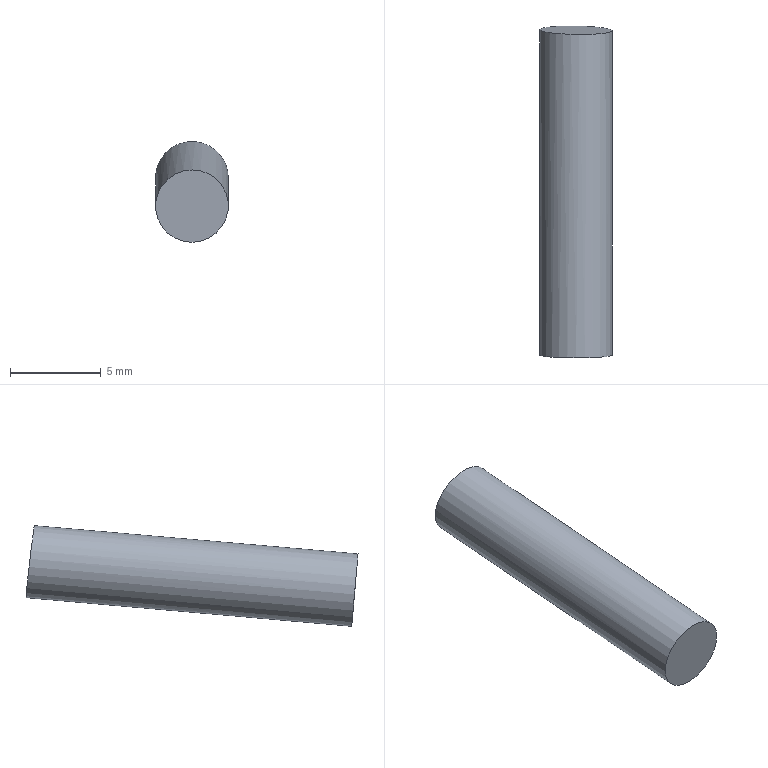Part | NX | features solid 2 | 1 solid | 3 faces | box 4 x 18.273 x 5.543 mm | volume 225.343 mm3 | plane 2 | cylinder 1 | commonest cylinder face diameters 4 x1
STEP:
#1=CARTESIAN_POINT('',(188.737,38.516,-31.599));
#2=VERTEX_POINT('',#1);
#3=CARTESIAN_POINT('',(188.737,38.342,-29.607));
#4=DIRECTION('',(0.,-0.9962,-0.08716));
#5=DIRECTION('',(0.,0.08716,-0.9962));
#6=AXIS2_PLACEMENT_3D('',#3,#4,#5);
#7=CIRCLE('',#6,2.);
#8=EDGE_CURVE('',#2,#2,#7,.T.);
#9=ORIENTED_EDGE('',*,*,#8,.T.);
#10=EDGE_LOOP('',(#9));
#11=FACE_BOUND('',#10,.T.);
#12=CARTESIAN_POINT('',(188.737,38.342,-29.607));
#13=DIRECTION('',(0.,-0.9962,-0.08716));
#14=DIRECTION('',(0.,-0.08716,0.9962));
#15=AXIS2_PLACEMENT_3D('',#12,#13,#14);
#16=PLANE('',#15);
#17=ADVANCED_FACE('',(#11),#16,.T.);
#18=CARTESIAN_POINT('',(189.678,55.986,-26.292));
#19=VERTEX_POINT('',#18);
#20=CARTESIAN_POINT('',(188.737,56.206,-28.044));
#21=DIRECTION('',(0.01549,0.9931,0.116));
#22=DIRECTION('',(0.4705,-0.1096,0.8755));
#23=AXIS2_PLACEMENT_3D('',#20,#21,#22);
#24=ELLIPSE('',#23,2.001,2.);
#25=EDGE_CURVE('',#19,#19,#24,.T.);
#26=ORIENTED_EDGE('',*,*,#25,.T.);
#27=EDGE_LOOP('',(#26));
#28=FACE_BOUND('',#27,.T.);
#29=CARTESIAN_POINT('',(159.246,62.921,-81.584));
#30=DIRECTION('',(0.01549,0.9931,0.116));
#31=DIRECTION('',(0.06594,-0.1168,0.991));
#32=AXIS2_PLACEMENT_3D('',#29,#30,#31);
#33=PLANE('',#32);
#34=ADVANCED_FACE('',(#28),#33,.T.);
#35=ORIENTED_EDGE('',*,*,#8,.F.);
#36=EDGE_LOOP('',(#35));
#37=FACE_BOUND('',#36,.T.);
#38=ORIENTED_EDGE('',*,*,#25,.F.);
#39=EDGE_LOOP('',(#38));
#40=FACE_BOUND('',#39,.T.);
#41=CARTESIAN_POINT('',(188.737,58.266,-27.864));
#42=DIRECTION('',(0.,-0.9962,-0.08716));
#43=DIRECTION('',(0.,-0.08716,0.9962));
#44=AXIS2_PLACEMENT_3D('',#41,#42,#43);
#45=CYLINDRICAL_SURFACE('',#44,2.);
#46=ADVANCED_FACE('',(#37,#40),#45,.T.);
#47=CLOSED_SHELL('',(#17,#34,#46));
#48=MANIFOLD_SOLID_BREP('',#47);
#49=(LENGTH_UNIT()NAMED_UNIT(*)SI_UNIT(.MILLI.,.METRE.));
#50=UNCERTAINTY_MEASURE_WITH_UNIT(LENGTH_MEASURE(0.00001),#49,'','');
#51=(NAMED_UNIT(*)PLANE_ANGLE_UNIT()SI_UNIT($,.RADIAN.));
#52=(NAMED_UNIT(*)SI_UNIT($,.STERADIAN.)SOLID_ANGLE_UNIT());
#53=(GEOMETRIC_REPRESENTATION_CONTEXT(3)GLOBAL_UNCERTAINTY_ASSIGNED_CONTEXT((#50))GLOBAL_UNIT_ASSIGNED_CONTEXT((#49,#51,#52))REPRESENTATION_CONTEXT('',''));
#54=ADVANCED_BREP_SHAPE_REPRESENTATION('',(#48),#53);